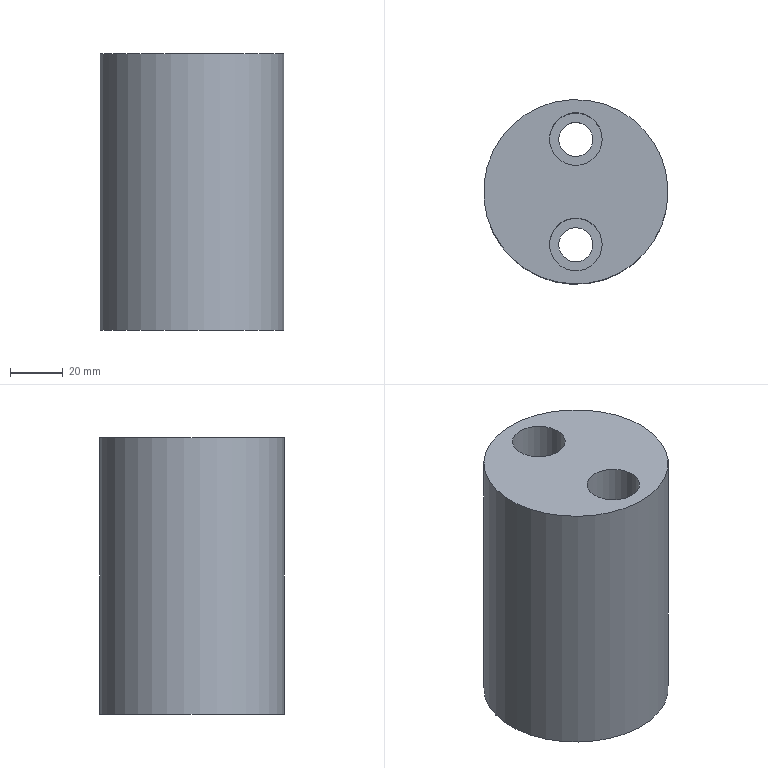Part | NX | features solid 2 | 1 solid | 9 faces | box 70 x 70 x 105 mm | volume 349000 mm3 | cylinder 5 | plane 4 | commonest cylinder face diameters 13 x2 20 x2 70 x1
STEP:
#1=CARTESIAN_POINT('',(-354.,440.,100.));
#2=VERTEX_POINT('',#1);
#3=CARTESIAN_POINT('',(-389.,440.,100.));
#4=DIRECTION('',(0.,0.,1.));
#5=DIRECTION('',(1.,0.,0.));
#6=AXIS2_PLACEMENT_3D('',#3,#4,#5);
#7=CIRCLE('',#6,35.);
#8=EDGE_CURVE('',#2,#2,#7,.T.);
#9=ORIENTED_EDGE('',*,*,#8,.T.);
#10=EDGE_LOOP('',(#9));
#11=FACE_BOUND('',#10,.T.);
#12=CARTESIAN_POINT('',(-354.,440.,205.));
#13=VERTEX_POINT('',#12);
#14=CARTESIAN_POINT('',(-389.,440.,205.));
#15=DIRECTION('',(0.,0.,1.));
#16=DIRECTION('',(1.,0.,0.));
#17=AXIS2_PLACEMENT_3D('',#14,#15,#16);
#18=CIRCLE('',#17,35.);
#19=EDGE_CURVE('',#13,#13,#18,.T.);
#20=ORIENTED_EDGE('',*,*,#19,.F.);
#21=EDGE_LOOP('',(#20));
#22=FACE_BOUND('',#21,.T.);
#23=CARTESIAN_POINT('',(-389.,440.,-95.));
#24=DIRECTION('',(0.,0.,1.));
#25=DIRECTION('',(1.,0.,0.));
#26=AXIS2_PLACEMENT_3D('',#23,#24,#25);
#27=CYLINDRICAL_SURFACE('',#26,35.);
#28=ADVANCED_FACE('',(#11,#22),#27,.T.);
#29=CARTESIAN_POINT('',(-382.5,420.,100.));
#30=VERTEX_POINT('',#29);
#31=CARTESIAN_POINT('',(-389.,420.,100.));
#32=DIRECTION('',(0.,0.,1.));
#33=DIRECTION('',(1.,0.,0.));
#34=AXIS2_PLACEMENT_3D('',#31,#32,#33);
#35=CIRCLE('',#34,6.5);
#36=EDGE_CURVE('',#30,#30,#35,.T.);
#37=ORIENTED_EDGE('',*,*,#36,.T.);
#38=EDGE_LOOP('',(#37));
#39=FACE_BOUND('',#38,.T.);
#40=CARTESIAN_POINT('',(-382.5,460.,100.));
#41=VERTEX_POINT('',#40);
#42=CARTESIAN_POINT('',(-389.,460.,100.));
#43=DIRECTION('',(0.,0.,1.));
#44=DIRECTION('',(1.,0.,0.));
#45=AXIS2_PLACEMENT_3D('',#42,#43,#44);
#46=CIRCLE('',#45,6.5);
#47=EDGE_CURVE('',#41,#41,#46,.T.);
#48=ORIENTED_EDGE('',*,*,#47,.T.);
#49=EDGE_LOOP('',(#48));
#50=FACE_BOUND('',#49,.T.);
#51=ORIENTED_EDGE('',*,*,#8,.F.);
#52=EDGE_LOOP('',(#51));
#53=FACE_BOUND('',#52,.T.);
#54=CARTESIAN_POINT('',(-389.,440.,100.));
#55=DIRECTION('',(0.,0.,1.));
#56=DIRECTION('',(1.,0.,0.));
#57=AXIS2_PLACEMENT_3D('',#54,#55,#56);
#58=PLANE('',#57);
#59=ADVANCED_FACE('',(#39,#50,#53),#58,.F.);
#60=CARTESIAN_POINT('',(-379.,420.,205.));
#61=VERTEX_POINT('',#60);
#62=CARTESIAN_POINT('',(-389.,420.,205.));
#63=DIRECTION('',(0.,0.,1.));
#64=DIRECTION('',(1.,0.,0.));
#65=AXIS2_PLACEMENT_3D('',#62,#63,#64);
#66=CIRCLE('',#65,10.);
#67=EDGE_CURVE('',#61,#61,#66,.T.);
#68=ORIENTED_EDGE('',*,*,#67,.F.);
#69=EDGE_LOOP('',(#68));
#70=FACE_BOUND('',#69,.T.);
#71=CARTESIAN_POINT('',(-379.,460.,205.));
#72=VERTEX_POINT('',#71);
#73=CARTESIAN_POINT('',(-389.,460.,205.));
#74=DIRECTION('',(0.,0.,1.));
#75=DIRECTION('',(1.,0.,0.));
#76=AXIS2_PLACEMENT_3D('',#73,#74,#75);
#77=CIRCLE('',#76,10.);
#78=EDGE_CURVE('',#72,#72,#77,.T.);
#79=ORIENTED_EDGE('',*,*,#78,.F.);
#80=EDGE_LOOP('',(#79));
#81=FACE_BOUND('',#80,.T.);
#82=ORIENTED_EDGE('',*,*,#19,.T.);
#83=EDGE_LOOP('',(#82));
#84=FACE_BOUND('',#83,.T.);
#85=CARTESIAN_POINT('',(-389.,440.,205.));
#86=DIRECTION('',(0.,0.,1.));
#87=DIRECTION('',(1.,0.,0.));
#88=AXIS2_PLACEMENT_3D('',#85,#86,#87);
#89=PLANE('',#88);
#90=ADVANCED_FACE('',(#70,#81,#84),#89,.T.);
#91=CARTESIAN_POINT('',(-395.5,460.,130.));
#92=VERTEX_POINT('',#91);
#93=CARTESIAN_POINT('',(-389.,460.,130.));
#94=DIRECTION('',(0.,0.,-1.));
#95=DIRECTION('',(-1.,0.,0.));
#96=AXIS2_PLACEMENT_3D('',#93,#94,#95);
#97=CIRCLE('',#96,6.5);
#98=EDGE_CURVE('',#92,#92,#97,.F.);
#99=ORIENTED_EDGE('',*,*,#98,.T.);
#100=EDGE_LOOP('',(#99));
#101=FACE_BOUND('',#100,.T.);
#102=ORIENTED_EDGE('',*,*,#47,.F.);
#103=EDGE_LOOP('',(#102));
#104=FACE_BOUND('',#103,.T.);
#105=CARTESIAN_POINT('',(-389.,460.,70.));
#106=DIRECTION('',(0.,0.,1.));
#107=DIRECTION('',(1.,0.,0.));
#108=AXIS2_PLACEMENT_3D('',#105,#106,#107);
#109=CYLINDRICAL_SURFACE('',#108,6.5);
#110=ADVANCED_FACE('',(#101,#104),#109,.F.);
#111=ORIENTED_EDGE('',*,*,#98,.F.);
#112=EDGE_LOOP('',(#111));
#113=FACE_BOUND('',#112,.T.);
#114=CARTESIAN_POINT('',(-379.,460.,130.));
#115=VERTEX_POINT('',#114);
#116=CARTESIAN_POINT('',(-389.,460.,130.));
#117=DIRECTION('',(0.,0.,1.));
#118=DIRECTION('',(1.,0.,0.));
#119=AXIS2_PLACEMENT_3D('',#116,#117,#118);
#120=CIRCLE('',#119,10.);
#121=EDGE_CURVE('',#115,#115,#120,.T.);
#122=ORIENTED_EDGE('',*,*,#121,.T.);
#123=EDGE_LOOP('',(#122));
#124=FACE_BOUND('',#123,.T.);
#125=CARTESIAN_POINT('',(-389.,460.,130.));
#126=DIRECTION('',(0.,0.,-1.));
#127=DIRECTION('',(-1.,0.,0.));
#128=AXIS2_PLACEMENT_3D('',#125,#126,#127);
#129=PLANE('',#128);
#130=ADVANCED_FACE('',(#113,#124),#129,.F.);
#131=ORIENTED_EDGE('',*,*,#78,.T.);
#132=EDGE_LOOP('',(#131));
#133=FACE_BOUND('',#132,.T.);
#134=ORIENTED_EDGE('',*,*,#121,.F.);
#135=EDGE_LOOP('',(#134));
#136=FACE_BOUND('',#135,.T.);
#137=CARTESIAN_POINT('',(-389.,460.,130.));
#138=DIRECTION('',(0.,0.,1.));
#139=DIRECTION('',(1.,0.,0.));
#140=AXIS2_PLACEMENT_3D('',#137,#138,#139);
#141=CYLINDRICAL_SURFACE('',#140,10.);
#142=ADVANCED_FACE('',(#133,#136),#141,.F.);
#143=CARTESIAN_POINT('',(-395.5,420.,130.));
#144=VERTEX_POINT('',#143);
#145=CARTESIAN_POINT('',(-389.,420.,130.));
#146=DIRECTION('',(0.,0.,-1.));
#147=DIRECTION('',(-1.,0.,0.));
#148=AXIS2_PLACEMENT_3D('',#145,#146,#147);
#149=CIRCLE('',#148,6.5);
#150=EDGE_CURVE('',#144,#144,#149,.F.);
#151=ORIENTED_EDGE('',*,*,#150,.T.);
#152=EDGE_LOOP('',(#151));
#153=FACE_BOUND('',#152,.T.);
#154=ORIENTED_EDGE('',*,*,#36,.F.);
#155=EDGE_LOOP('',(#154));
#156=FACE_BOUND('',#155,.T.);
#157=CARTESIAN_POINT('',(-389.,420.,70.));
#158=DIRECTION('',(0.,0.,1.));
#159=DIRECTION('',(1.,0.,0.));
#160=AXIS2_PLACEMENT_3D('',#157,#158,#159);
#161=CYLINDRICAL_SURFACE('',#160,6.5);
#162=ADVANCED_FACE('',(#153,#156),#161,.F.);
#163=ORIENTED_EDGE('',*,*,#150,.F.);
#164=EDGE_LOOP('',(#163));
#165=FACE_BOUND('',#164,.T.);
#166=CARTESIAN_POINT('',(-379.,420.,130.));
#167=VERTEX_POINT('',#166);
#168=CARTESIAN_POINT('',(-389.,420.,130.));
#169=DIRECTION('',(0.,0.,1.));
#170=DIRECTION('',(1.,0.,0.));
#171=AXIS2_PLACEMENT_3D('',#168,#169,#170);
#172=CIRCLE('',#171,10.);
#173=EDGE_CURVE('',#167,#167,#172,.T.);
#174=ORIENTED_EDGE('',*,*,#173,.T.);
#175=EDGE_LOOP('',(#174));
#176=FACE_BOUND('',#175,.T.);
#177=CARTESIAN_POINT('',(-389.,420.,130.));
#178=DIRECTION('',(0.,0.,-1.));
#179=DIRECTION('',(-1.,0.,0.));
#180=AXIS2_PLACEMENT_3D('',#177,#178,#179);
#181=PLANE('',#180);
#182=ADVANCED_FACE('',(#165,#176),#181,.F.);
#183=ORIENTED_EDGE('',*,*,#67,.T.);
#184=EDGE_LOOP('',(#183));
#185=FACE_BOUND('',#184,.T.);
#186=ORIENTED_EDGE('',*,*,#173,.F.);
#187=EDGE_LOOP('',(#186));
#188=FACE_BOUND('',#187,.T.);
#189=CARTESIAN_POINT('',(-389.,420.,130.));
#190=DIRECTION('',(0.,0.,1.));
#191=DIRECTION('',(1.,0.,0.));
#192=AXIS2_PLACEMENT_3D('',#189,#190,#191);
#193=CYLINDRICAL_SURFACE('',#192,10.);
#194=ADVANCED_FACE('',(#185,#188),#193,.F.);
#195=CLOSED_SHELL('',(#28,#59,#90,#110,#130,#142,#162,#182,#194));
#196=MANIFOLD_SOLID_BREP('',#195);
#197=(LENGTH_UNIT()NAMED_UNIT(*)SI_UNIT(.MILLI.,.METRE.));
#198=UNCERTAINTY_MEASURE_WITH_UNIT(LENGTH_MEASURE(0.00001),#197,'','');
#199=(NAMED_UNIT(*)PLANE_ANGLE_UNIT()SI_UNIT($,.RADIAN.));
#200=(NAMED_UNIT(*)SI_UNIT($,.STERADIAN.)SOLID_ANGLE_UNIT());
#201=(GEOMETRIC_REPRESENTATION_CONTEXT(3)GLOBAL_UNCERTAINTY_ASSIGNED_CONTEXT((#198))GLOBAL_UNIT_ASSIGNED_CONTEXT((#197,#199,#200))REPRESENTATION_CONTEXT('',''));
#202=ADVANCED_BREP_SHAPE_REPRESENTATION('',(#196),#201);